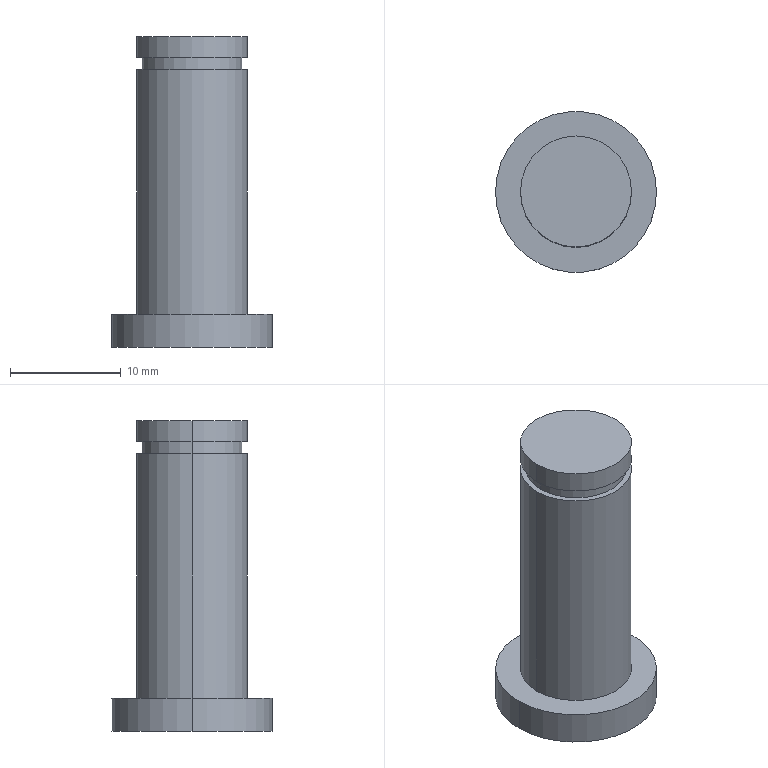Part | NX | features BREP 1 | 1 solid | 13 faces | box 14.5 x 14.5 x 28 mm | volume 2442 mm3 | cylinder 8 | plane 5 | commonest cylinder face diameters 10 x4 9 x2 14.5 x2
STEP:
#1=CARTESIAN_POINT('',(5.,0.,28.));
#2=VERTEX_POINT('',#1);
#3=CARTESIAN_POINT('',(-5.,0.,28.));
#4=VERTEX_POINT('',#3);
#5=CARTESIAN_POINT('',(0.,0.,28.));
#6=DIRECTION('',(0.,0.,1.));
#7=DIRECTION('',(1.,0.,0.));
#8=AXIS2_PLACEMENT_3D('',#5,#6,#7);
#9=CIRCLE('',#8,5.);
#10=EDGE_CURVE('',#2,#4,#9,.T.);
#11=ORIENTED_EDGE('',*,*,#10,.F.);
#12=CARTESIAN_POINT('',(5.,0.,26.1));
#13=VERTEX_POINT('',#12);
#14=CARTESIAN_POINT('',(5.,0.,28.));
#15=DIRECTION('',(0.,0.,-1.));
#16=VECTOR('',#15,1000.);
#17=LINE('',#14,#16);
#18=EDGE_CURVE('',#2,#13,#17,.T.);
#19=ORIENTED_EDGE('',*,*,#18,.T.);
#20=CARTESIAN_POINT('',(-5.,0.,26.1));
#21=VERTEX_POINT('',#20);
#22=CARTESIAN_POINT('',(0.,0.,26.1));
#23=DIRECTION('',(0.,0.,1.));
#24=DIRECTION('',(1.,0.,0.));
#25=AXIS2_PLACEMENT_3D('',#22,#23,#24);
#26=CIRCLE('',#25,5.);
#27=EDGE_CURVE('',#13,#21,#26,.T.);
#28=ORIENTED_EDGE('',*,*,#27,.T.);
#29=CARTESIAN_POINT('',(-5.,0.,28.));
#30=DIRECTION('',(0.,0.,-1.));
#31=VECTOR('',#30,1000.);
#32=LINE('',#29,#31);
#33=EDGE_CURVE('',#4,#21,#32,.T.);
#34=ORIENTED_EDGE('',*,*,#33,.F.);
#35=EDGE_LOOP('',(#11,#19,#28,#34));
#36=FACE_BOUND('',#35,.T.);
#37=CARTESIAN_POINT('',(0.,0.,28.));
#38=DIRECTION('',(0.,0.,-1.));
#39=DIRECTION('',(-1.,0.,0.));
#40=AXIS2_PLACEMENT_3D('',#37,#38,#39);
#41=CYLINDRICAL_SURFACE('',#40,5.);
#42=ADVANCED_FACE('',(#36),#41,.T.);
#43=CARTESIAN_POINT('',(4.5,0.,26.1));
#44=VERTEX_POINT('',#43);
#45=CARTESIAN_POINT('',(-4.5,0.,26.1));
#46=VERTEX_POINT('',#45);
#47=CARTESIAN_POINT('',(0.,0.,26.1));
#48=DIRECTION('',(0.,0.,1.));
#49=DIRECTION('',(1.,0.,0.));
#50=AXIS2_PLACEMENT_3D('',#47,#48,#49);
#51=CIRCLE('',#50,4.5);
#52=EDGE_CURVE('',#44,#46,#51,.T.);
#53=ORIENTED_EDGE('',*,*,#52,.F.);
#54=CARTESIAN_POINT('',(4.5,0.,25.));
#55=VERTEX_POINT('',#54);
#56=CARTESIAN_POINT('',(4.5,0.,26.1));
#57=DIRECTION('',(0.,0.,-1.));
#58=VECTOR('',#57,1000.);
#59=LINE('',#56,#58);
#60=EDGE_CURVE('',#44,#55,#59,.T.);
#61=ORIENTED_EDGE('',*,*,#60,.T.);
#62=CARTESIAN_POINT('',(-4.5,0.,25.));
#63=VERTEX_POINT('',#62);
#64=CARTESIAN_POINT('',(0.,0.,25.));
#65=DIRECTION('',(0.,0.,1.));
#66=DIRECTION('',(1.,0.,0.));
#67=AXIS2_PLACEMENT_3D('',#64,#65,#66);
#68=CIRCLE('',#67,4.5);
#69=EDGE_CURVE('',#55,#63,#68,.T.);
#70=ORIENTED_EDGE('',*,*,#69,.T.);
#71=CARTESIAN_POINT('',(-4.5,0.,26.1));
#72=DIRECTION('',(0.,0.,-1.));
#73=VECTOR('',#72,1000.);
#74=LINE('',#71,#73);
#75=EDGE_CURVE('',#46,#63,#74,.T.);
#76=ORIENTED_EDGE('',*,*,#75,.F.);
#77=EDGE_LOOP('',(#53,#61,#70,#76));
#78=FACE_BOUND('',#77,.T.);
#79=CARTESIAN_POINT('',(0.,0.,26.1));
#80=DIRECTION('',(0.,0.,-1.));
#81=DIRECTION('',(-1.,0.,0.));
#82=AXIS2_PLACEMENT_3D('',#79,#80,#81);
#83=CYLINDRICAL_SURFACE('',#82,4.5);
#84=ADVANCED_FACE('',(#78),#83,.T.);
#85=CARTESIAN_POINT('',(7.25,0.,3.));
#86=VERTEX_POINT('',#85);
#87=CARTESIAN_POINT('',(-7.25,0.,3.));
#88=VERTEX_POINT('',#87);
#89=CARTESIAN_POINT('',(0.,0.,3.));
#90=DIRECTION('',(0.,0.,1.));
#91=DIRECTION('',(1.,0.,0.));
#92=AXIS2_PLACEMENT_3D('',#89,#90,#91);
#93=CIRCLE('',#92,7.25);
#94=EDGE_CURVE('',#86,#88,#93,.T.);
#95=ORIENTED_EDGE('',*,*,#94,.F.);
#96=CARTESIAN_POINT('',(7.25,0.,0.));
#97=VERTEX_POINT('',#96);
#98=CARTESIAN_POINT('',(7.25,0.,3.));
#99=DIRECTION('',(0.,0.,-1.));
#100=VECTOR('',#99,1000.);
#101=LINE('',#98,#100);
#102=EDGE_CURVE('',#86,#97,#101,.T.);
#103=ORIENTED_EDGE('',*,*,#102,.T.);
#104=CARTESIAN_POINT('',(-7.25,0.,0.));
#105=VERTEX_POINT('',#104);
#106=CARTESIAN_POINT('',(0.,0.,0.));
#107=DIRECTION('',(0.,0.,1.));
#108=DIRECTION('',(1.,0.,0.));
#109=AXIS2_PLACEMENT_3D('',#106,#107,#108);
#110=CIRCLE('',#109,7.25);
#111=EDGE_CURVE('',#97,#105,#110,.T.);
#112=ORIENTED_EDGE('',*,*,#111,.T.);
#113=CARTESIAN_POINT('',(-7.25,0.,3.));
#114=DIRECTION('',(0.,0.,-1.));
#115=VECTOR('',#114,1000.);
#116=LINE('',#113,#115);
#117=EDGE_CURVE('',#88,#105,#116,.T.);
#118=ORIENTED_EDGE('',*,*,#117,.F.);
#119=EDGE_LOOP('',(#95,#103,#112,#118));
#120=FACE_BOUND('',#119,.T.);
#121=CARTESIAN_POINT('',(0.,0.,3.));
#122=DIRECTION('',(0.,0.,-1.));
#123=DIRECTION('',(-1.,0.,0.));
#124=AXIS2_PLACEMENT_3D('',#121,#122,#123);
#125=CYLINDRICAL_SURFACE('',#124,7.25);
#126=ADVANCED_FACE('',(#120),#125,.T.);
#127=CARTESIAN_POINT('',(5.,0.,25.));
#128=VERTEX_POINT('',#127);
#129=CARTESIAN_POINT('',(-5.,0.,25.));
#130=VERTEX_POINT('',#129);
#131=CARTESIAN_POINT('',(0.,0.,25.));
#132=DIRECTION('',(0.,0.,1.));
#133=DIRECTION('',(1.,0.,0.));
#134=AXIS2_PLACEMENT_3D('',#131,#132,#133);
#135=CIRCLE('',#134,5.);
#136=EDGE_CURVE('',#128,#130,#135,.T.);
#137=ORIENTED_EDGE('',*,*,#136,.F.);
#138=CARTESIAN_POINT('',(5.,0.,3.));
#139=VERTEX_POINT('',#138);
#140=CARTESIAN_POINT('',(5.,0.,28.));
#141=DIRECTION('',(0.,0.,-1.));
#142=VECTOR('',#141,1000.);
#143=LINE('',#140,#142);
#144=EDGE_CURVE('',#128,#139,#143,.T.);
#145=ORIENTED_EDGE('',*,*,#144,.T.);
#146=CARTESIAN_POINT('',(-5.,0.,3.));
#147=VERTEX_POINT('',#146);
#148=CARTESIAN_POINT('',(0.,0.,3.));
#149=DIRECTION('',(0.,0.,1.));
#150=DIRECTION('',(1.,0.,0.));
#151=AXIS2_PLACEMENT_3D('',#148,#149,#150);
#152=CIRCLE('',#151,5.);
#153=EDGE_CURVE('',#139,#147,#152,.T.);
#154=ORIENTED_EDGE('',*,*,#153,.T.);
#155=CARTESIAN_POINT('',(-5.,0.,28.));
#156=DIRECTION('',(0.,0.,-1.));
#157=VECTOR('',#156,1000.);
#158=LINE('',#155,#157);
#159=EDGE_CURVE('',#130,#147,#158,.T.);
#160=ORIENTED_EDGE('',*,*,#159,.F.);
#161=EDGE_LOOP('',(#137,#145,#154,#160));
#162=FACE_BOUND('',#161,.T.);
#163=CARTESIAN_POINT('',(0.,0.,28.));
#164=DIRECTION('',(0.,0.,-1.));
#165=DIRECTION('',(-1.,0.,0.));
#166=AXIS2_PLACEMENT_3D('',#163,#164,#165);
#167=CYLINDRICAL_SURFACE('',#166,5.);
#168=ADVANCED_FACE('',(#162),#167,.T.);
#169=ORIENTED_EDGE('',*,*,#144,.F.);
#170=CARTESIAN_POINT('',(0.,0.,25.));
#171=DIRECTION('',(0.,0.,1.));
#172=DIRECTION('',(1.,0.,0.));
#173=AXIS2_PLACEMENT_3D('',#170,#171,#172);
#174=CIRCLE('',#173,5.);
#175=EDGE_CURVE('',#130,#128,#174,.T.);
#176=ORIENTED_EDGE('',*,*,#175,.F.);
#177=ORIENTED_EDGE('',*,*,#159,.T.);
#178=CARTESIAN_POINT('',(0.,0.,3.));
#179=DIRECTION('',(0.,0.,1.));
#180=DIRECTION('',(1.,0.,0.));
#181=AXIS2_PLACEMENT_3D('',#178,#179,#180);
#182=CIRCLE('',#181,5.);
#183=EDGE_CURVE('',#147,#139,#182,.T.);
#184=ORIENTED_EDGE('',*,*,#183,.T.);
#185=EDGE_LOOP('',(#169,#176,#177,#184));
#186=FACE_BOUND('',#185,.T.);
#187=CARTESIAN_POINT('',(0.,0.,28.));
#188=DIRECTION('',(0.,0.,-1.));
#189=DIRECTION('',(-1.,0.,0.));
#190=AXIS2_PLACEMENT_3D('',#187,#188,#189);
#191=CYLINDRICAL_SURFACE('',#190,5.);
#192=ADVANCED_FACE('',(#186),#191,.T.);
#193=ORIENTED_EDGE('',*,*,#102,.F.);
#194=CARTESIAN_POINT('',(0.,0.,3.));
#195=DIRECTION('',(0.,0.,1.));
#196=DIRECTION('',(1.,0.,0.));
#197=AXIS2_PLACEMENT_3D('',#194,#195,#196);
#198=CIRCLE('',#197,7.25);
#199=EDGE_CURVE('',#88,#86,#198,.T.);
#200=ORIENTED_EDGE('',*,*,#199,.F.);
#201=ORIENTED_EDGE('',*,*,#117,.T.);
#202=CARTESIAN_POINT('',(0.,0.,0.));
#203=DIRECTION('',(0.,0.,1.));
#204=DIRECTION('',(1.,0.,0.));
#205=AXIS2_PLACEMENT_3D('',#202,#203,#204);
#206=CIRCLE('',#205,7.25);
#207=EDGE_CURVE('',#105,#97,#206,.T.);
#208=ORIENTED_EDGE('',*,*,#207,.T.);
#209=EDGE_LOOP('',(#193,#200,#201,#208));
#210=FACE_BOUND('',#209,.T.);
#211=CARTESIAN_POINT('',(0.,0.,3.));
#212=DIRECTION('',(0.,0.,-1.));
#213=DIRECTION('',(-1.,0.,0.));
#214=AXIS2_PLACEMENT_3D('',#211,#212,#213);
#215=CYLINDRICAL_SURFACE('',#214,7.25);
#216=ADVANCED_FACE('',(#210),#215,.T.);
#217=ORIENTED_EDGE('',*,*,#199,.T.);
#218=ORIENTED_EDGE('',*,*,#94,.T.);
#219=EDGE_LOOP('',(#217,#218));
#220=FACE_BOUND('',#219,.T.);
#221=ORIENTED_EDGE('',*,*,#183,.F.);
#222=ORIENTED_EDGE('',*,*,#153,.F.);
#223=EDGE_LOOP('',(#221,#222));
#224=FACE_BOUND('',#223,.T.);
#225=CARTESIAN_POINT('',(0.,0.,3.));
#226=DIRECTION('',(0.,0.,1.));
#227=DIRECTION('',(1.,0.,0.));
#228=AXIS2_PLACEMENT_3D('',#225,#226,#227);
#229=PLANE('',#228);
#230=ADVANCED_FACE('',(#220,#224),#229,.T.);
#231=ORIENTED_EDGE('',*,*,#207,.F.);
#232=ORIENTED_EDGE('',*,*,#111,.F.);
#233=EDGE_LOOP('',(#231,#232));
#234=FACE_BOUND('',#233,.T.);
#235=CARTESIAN_POINT('',(0.,0.,0.));
#236=DIRECTION('',(0.,0.,1.));
#237=DIRECTION('',(1.,0.,0.));
#238=AXIS2_PLACEMENT_3D('',#235,#236,#237);
#239=PLANE('',#238);
#240=ADVANCED_FACE('',(#234),#239,.F.);
#241=CARTESIAN_POINT('',(0.,0.,26.1));
#242=DIRECTION('',(0.,0.,1.));
#243=DIRECTION('',(1.,0.,0.));
#244=AXIS2_PLACEMENT_3D('',#241,#242,#243);
#245=CIRCLE('',#244,5.);
#246=EDGE_CURVE('',#21,#13,#245,.T.);
#247=ORIENTED_EDGE('',*,*,#246,.F.);
#248=ORIENTED_EDGE('',*,*,#27,.F.);
#249=EDGE_LOOP('',(#247,#248));
#250=FACE_BOUND('',#249,.T.);
#251=CARTESIAN_POINT('',(0.,0.,26.1));
#252=DIRECTION('',(0.,0.,1.));
#253=DIRECTION('',(1.,0.,0.));
#254=AXIS2_PLACEMENT_3D('',#251,#252,#253);
#255=CIRCLE('',#254,4.5);
#256=EDGE_CURVE('',#46,#44,#255,.T.);
#257=ORIENTED_EDGE('',*,*,#256,.T.);
#258=ORIENTED_EDGE('',*,*,#52,.T.);
#259=EDGE_LOOP('',(#257,#258));
#260=FACE_BOUND('',#259,.T.);
#261=CARTESIAN_POINT('',(0.,0.,26.1));
#262=DIRECTION('',(0.,0.,1.));
#263=DIRECTION('',(1.,0.,0.));
#264=AXIS2_PLACEMENT_3D('',#261,#262,#263);
#265=PLANE('',#264);
#266=ADVANCED_FACE('',(#250,#260),#265,.F.);
#267=ORIENTED_EDGE('',*,*,#175,.T.);
#268=ORIENTED_EDGE('',*,*,#136,.T.);
#269=EDGE_LOOP('',(#267,#268));
#270=FACE_BOUND('',#269,.T.);
#271=CARTESIAN_POINT('',(0.,0.,25.));
#272=DIRECTION('',(0.,0.,1.));
#273=DIRECTION('',(1.,0.,0.));
#274=AXIS2_PLACEMENT_3D('',#271,#272,#273);
#275=CIRCLE('',#274,4.5);
#276=EDGE_CURVE('',#63,#55,#275,.T.);
#277=ORIENTED_EDGE('',*,*,#276,.F.);
#278=ORIENTED_EDGE('',*,*,#69,.F.);
#279=EDGE_LOOP('',(#277,#278));
#280=FACE_BOUND('',#279,.T.);
#281=CARTESIAN_POINT('',(0.,0.,25.));
#282=DIRECTION('',(0.,0.,1.));
#283=DIRECTION('',(1.,0.,0.));
#284=AXIS2_PLACEMENT_3D('',#281,#282,#283);
#285=PLANE('',#284);
#286=ADVANCED_FACE('',(#270,#280),#285,.T.);
#287=ORIENTED_EDGE('',*,*,#60,.F.);
#288=ORIENTED_EDGE('',*,*,#256,.F.);
#289=ORIENTED_EDGE('',*,*,#75,.T.);
#290=ORIENTED_EDGE('',*,*,#276,.T.);
#291=EDGE_LOOP('',(#287,#288,#289,#290));
#292=FACE_BOUND('',#291,.T.);
#293=CARTESIAN_POINT('',(0.,0.,26.1));
#294=DIRECTION('',(0.,0.,-1.));
#295=DIRECTION('',(-1.,0.,0.));
#296=AXIS2_PLACEMENT_3D('',#293,#294,#295);
#297=CYLINDRICAL_SURFACE('',#296,4.5);
#298=ADVANCED_FACE('',(#292),#297,.T.);
#299=CARTESIAN_POINT('',(0.,0.,28.));
#300=DIRECTION('',(0.,0.,1.));
#301=DIRECTION('',(1.,0.,0.));
#302=AXIS2_PLACEMENT_3D('',#299,#300,#301);
#303=CIRCLE('',#302,5.);
#304=EDGE_CURVE('',#4,#2,#303,.T.);
#305=ORIENTED_EDGE('',*,*,#304,.T.);
#306=ORIENTED_EDGE('',*,*,#10,.T.);
#307=EDGE_LOOP('',(#305,#306));
#308=FACE_BOUND('',#307,.T.);
#309=CARTESIAN_POINT('',(0.,0.,28.));
#310=DIRECTION('',(0.,0.,1.));
#311=DIRECTION('',(1.,0.,0.));
#312=AXIS2_PLACEMENT_3D('',#309,#310,#311);
#313=PLANE('',#312);
#314=ADVANCED_FACE('',(#308),#313,.T.);
#315=ORIENTED_EDGE('',*,*,#18,.F.);
#316=ORIENTED_EDGE('',*,*,#304,.F.);
#317=ORIENTED_EDGE('',*,*,#33,.T.);
#318=ORIENTED_EDGE('',*,*,#246,.T.);
#319=EDGE_LOOP('',(#315,#316,#317,#318));
#320=FACE_BOUND('',#319,.T.);
#321=CARTESIAN_POINT('',(0.,0.,28.));
#322=DIRECTION('',(0.,0.,-1.));
#323=DIRECTION('',(-1.,0.,0.));
#324=AXIS2_PLACEMENT_3D('',#321,#322,#323);
#325=CYLINDRICAL_SURFACE('',#324,5.);
#326=ADVANCED_FACE('',(#320),#325,.T.);
#327=CLOSED_SHELL('',(#42,#84,#126,#168,#192,#216,#230,#240,#266,#286,#298,#314,#326));
#328=MANIFOLD_SOLID_BREP('',#327);
#329=(LENGTH_UNIT()NAMED_UNIT(*)SI_UNIT(.MILLI.,.METRE.));
#330=UNCERTAINTY_MEASURE_WITH_UNIT(LENGTH_MEASURE(0.00001),#329,'','');
#331=(NAMED_UNIT(*)PLANE_ANGLE_UNIT()SI_UNIT($,.RADIAN.));
#332=(NAMED_UNIT(*)SI_UNIT($,.STERADIAN.)SOLID_ANGLE_UNIT());
#333=(GEOMETRIC_REPRESENTATION_CONTEXT(3)GLOBAL_UNCERTAINTY_ASSIGNED_CONTEXT((#330))GLOBAL_UNIT_ASSIGNED_CONTEXT((#329,#331,#332))REPRESENTATION_CONTEXT('',''));
#334=ADVANCED_BREP_SHAPE_REPRESENTATION('',(#328),#333);